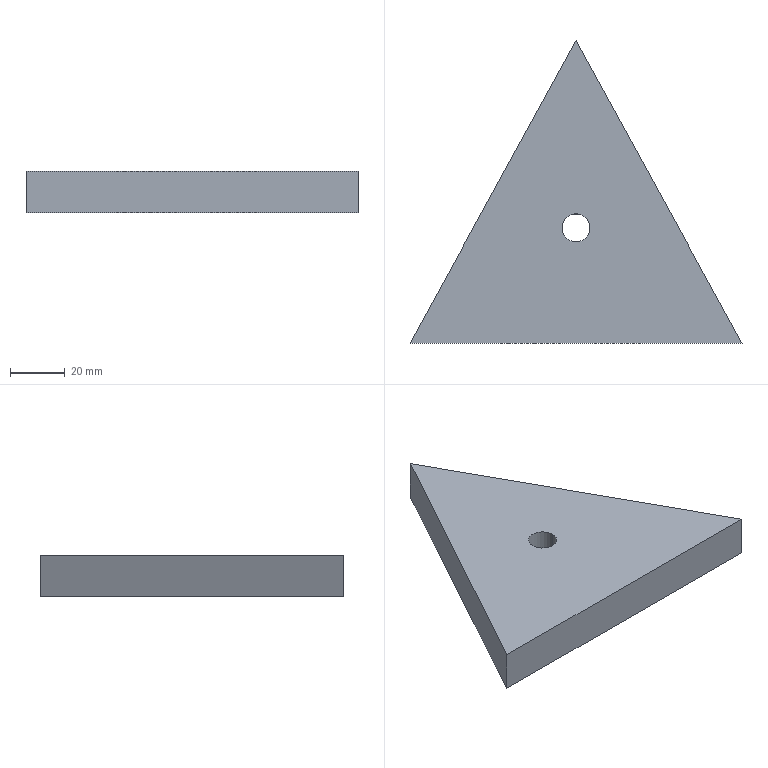Part | SolidWorks | features Extrusion 1, HoleWzd 1 | 1 solid | 7 faces | box 121 x 110.14 x 15 mm | volume 98726 mm3 | plane 5 | cylinder 2 | commonest cylinder face diameters 10.2 x2
STEP:
#1=CARTESIAN_POINT('',(5.1,-68.14,0.));
#2=VERTEX_POINT('',#1);
#3=CARTESIAN_POINT('',(-5.1,-68.14,0.));
#4=VERTEX_POINT('',#3);
#5=CARTESIAN_POINT('',(0.,-68.14,0.));
#6=DIRECTION('',(0.,0.,-1.));
#7=DIRECTION('',(-1.,0.,0.));
#8=AXIS2_PLACEMENT_3D('',#5,#6,#7);
#9=CIRCLE('',#8,5.1);
#10=EDGE_CURVE('',#2,#4,#9,.T.);
#11=ORIENTED_EDGE('',*,*,#10,.T.);
#12=CARTESIAN_POINT('',(-5.1,-68.14,15.));
#13=VERTEX_POINT('',#12);
#14=CARTESIAN_POINT('',(-5.1,-68.14,15.));
#15=DIRECTION('',(0.,0.,1.));
#16=VECTOR('',#15,1000.);
#17=LINE('',#14,#16);
#18=EDGE_CURVE('',#4,#13,#17,.T.);
#19=ORIENTED_EDGE('',*,*,#18,.T.);
#20=CARTESIAN_POINT('',(5.1,-68.14,15.));
#21=VERTEX_POINT('',#20);
#22=CARTESIAN_POINT('',(0.,-68.14,15.));
#23=DIRECTION('',(0.,0.,1.));
#24=DIRECTION('',(1.,0.,0.));
#25=AXIS2_PLACEMENT_3D('',#22,#23,#24);
#26=CIRCLE('',#25,5.1);
#27=EDGE_CURVE('',#13,#21,#26,.T.);
#28=ORIENTED_EDGE('',*,*,#27,.T.);
#29=CARTESIAN_POINT('',(5.1,-68.14,15.));
#30=DIRECTION('',(0.,0.,1.));
#31=VECTOR('',#30,1000.);
#32=LINE('',#29,#31);
#33=EDGE_CURVE('',#2,#21,#32,.T.);
#34=ORIENTED_EDGE('',*,*,#33,.F.);
#35=EDGE_LOOP('',(#11,#19,#28,#34));
#36=FACE_OUTER_BOUND('',#35,.T.);
#37=CARTESIAN_POINT('',(0.,-68.14,15.));
#38=DIRECTION('',(0.,0.,1.));
#39=DIRECTION('',(1.,0.,0.));
#40=AXIS2_PLACEMENT_3D('',#37,#38,#39);
#41=CYLINDRICAL_SURFACE('',#40,5.1);
#42=ADVANCED_FACE('',(#36),#41,.F.);
#43=CARTESIAN_POINT('',(0.,-68.14,15.));
#44=DIRECTION('',(0.,0.,1.));
#45=DIRECTION('',(1.,0.,0.));
#46=AXIS2_PLACEMENT_3D('',#43,#44,#45);
#47=CIRCLE('',#46,5.1);
#48=EDGE_CURVE('',#21,#13,#47,.T.);
#49=ORIENTED_EDGE('',*,*,#48,.F.);
#50=ORIENTED_EDGE('',*,*,#27,.F.);
#51=EDGE_LOOP('',(#49,#50));
#52=FACE_BOUND('',#51,.T.);
#53=CARTESIAN_POINT('',(60.5,-110.14,15.));
#54=VERTEX_POINT('',#53);
#55=CARTESIAN_POINT('',(0.,0.,15.));
#56=VERTEX_POINT('',#55);
#57=CARTESIAN_POINT('',(60.5,-110.14,15.));
#58=DIRECTION('',(-0.4814,0.8765,0.));
#59=VECTOR('',#58,1000.);
#60=LINE('',#57,#59);
#61=EDGE_CURVE('',#54,#56,#60,.T.);
#62=ORIENTED_EDGE('',*,*,#61,.T.);
#63=CARTESIAN_POINT('',(-60.5,-110.14,15.));
#64=VERTEX_POINT('',#63);
#65=CARTESIAN_POINT('',(0.,0.,15.));
#66=DIRECTION('',(-0.4814,-0.8765,0.));
#67=VECTOR('',#66,1000.);
#68=LINE('',#65,#67);
#69=EDGE_CURVE('',#56,#64,#68,.T.);
#70=ORIENTED_EDGE('',*,*,#69,.T.);
#71=CARTESIAN_POINT('',(-60.5,-110.14,15.));
#72=DIRECTION('',(1.,0.,0.));
#73=VECTOR('',#72,1000.);
#74=LINE('',#71,#73);
#75=EDGE_CURVE('',#64,#54,#74,.T.);
#76=ORIENTED_EDGE('',*,*,#75,.T.);
#77=EDGE_LOOP('',(#62,#70,#76));
#78=FACE_OUTER_BOUND('',#77,.T.);
#79=CARTESIAN_POINT('',(0.,0.,15.));
#80=DIRECTION('',(0.,0.,-1.));
#81=DIRECTION('',(-1.,0.,0.));
#82=AXIS2_PLACEMENT_3D('',#79,#80,#81);
#83=PLANE('',#82);
#84=ADVANCED_FACE('',(#52,#78),#83,.F.);
#85=ORIENTED_EDGE('',*,*,#10,.F.);
#86=CARTESIAN_POINT('',(0.,-68.14,0.));
#87=DIRECTION('',(0.,0.,-1.));
#88=DIRECTION('',(-1.,0.,0.));
#89=AXIS2_PLACEMENT_3D('',#86,#87,#88);
#90=CIRCLE('',#89,5.1);
#91=EDGE_CURVE('',#4,#2,#90,.T.);
#92=ORIENTED_EDGE('',*,*,#91,.F.);
#93=EDGE_LOOP('',(#85,#92));
#94=FACE_BOUND('',#93,.T.);
#95=CARTESIAN_POINT('',(60.5,-110.14,0.));
#96=VERTEX_POINT('',#95);
#97=CARTESIAN_POINT('',(0.,0.,0.));
#98=VERTEX_POINT('',#97);
#99=CARTESIAN_POINT('',(60.5,-110.14,0.));
#100=DIRECTION('',(-0.4814,0.8765,0.));
#101=VECTOR('',#100,1000.);
#102=LINE('',#99,#101);
#103=EDGE_CURVE('',#96,#98,#102,.T.);
#104=ORIENTED_EDGE('',*,*,#103,.F.);
#105=CARTESIAN_POINT('',(-60.5,-110.14,0.));
#106=VERTEX_POINT('',#105);
#107=CARTESIAN_POINT('',(-60.5,-110.14,0.));
#108=DIRECTION('',(1.,0.,0.));
#109=VECTOR('',#108,1000.);
#110=LINE('',#107,#109);
#111=EDGE_CURVE('',#106,#96,#110,.T.);
#112=ORIENTED_EDGE('',*,*,#111,.F.);
#113=CARTESIAN_POINT('',(0.,0.,0.));
#114=DIRECTION('',(-0.4814,-0.8765,0.));
#115=VECTOR('',#114,1000.);
#116=LINE('',#113,#115);
#117=EDGE_CURVE('',#98,#106,#116,.T.);
#118=ORIENTED_EDGE('',*,*,#117,.F.);
#119=EDGE_LOOP('',(#104,#112,#118));
#120=FACE_OUTER_BOUND('',#119,.T.);
#121=CARTESIAN_POINT('',(0.,0.,0.));
#122=DIRECTION('',(0.,0.,-1.));
#123=DIRECTION('',(-1.,0.,0.));
#124=AXIS2_PLACEMENT_3D('',#121,#122,#123);
#125=PLANE('',#124);
#126=ADVANCED_FACE('',(#94,#120),#125,.T.);
#127=ORIENTED_EDGE('',*,*,#103,.T.);
#128=CARTESIAN_POINT('',(0.,0.,15.));
#129=DIRECTION('',(0.,0.,-1.));
#130=VECTOR('',#129,1000.);
#131=LINE('',#128,#130);
#132=EDGE_CURVE('',#56,#98,#131,.T.);
#133=ORIENTED_EDGE('',*,*,#132,.F.);
#134=ORIENTED_EDGE('',*,*,#61,.F.);
#135=CARTESIAN_POINT('',(60.5,-110.14,15.));
#136=DIRECTION('',(0.,0.,-1.));
#137=VECTOR('',#136,1000.);
#138=LINE('',#135,#137);
#139=EDGE_CURVE('',#54,#96,#138,.T.);
#140=ORIENTED_EDGE('',*,*,#139,.T.);
#141=EDGE_LOOP('',(#127,#133,#134,#140));
#142=FACE_OUTER_BOUND('',#141,.T.);
#143=CARTESIAN_POINT('',(60.5,-110.14,15.));
#144=DIRECTION('',(-0.8765,-0.4814,0.));
#145=DIRECTION('',(0.4814,-0.8765,0.));
#146=AXIS2_PLACEMENT_3D('',#143,#144,#145);
#147=PLANE('',#146);
#148=ADVANCED_FACE('',(#142),#147,.F.);
#149=ORIENTED_EDGE('',*,*,#117,.T.);
#150=CARTESIAN_POINT('',(-60.5,-110.14,15.));
#151=DIRECTION('',(0.,0.,-1.));
#152=VECTOR('',#151,1000.);
#153=LINE('',#150,#152);
#154=EDGE_CURVE('',#64,#106,#153,.T.);
#155=ORIENTED_EDGE('',*,*,#154,.F.);
#156=ORIENTED_EDGE('',*,*,#69,.F.);
#157=ORIENTED_EDGE('',*,*,#132,.T.);
#158=EDGE_LOOP('',(#149,#155,#156,#157));
#159=FACE_OUTER_BOUND('',#158,.T.);
#160=CARTESIAN_POINT('',(0.,0.,15.));
#161=DIRECTION('',(0.8765,-0.4814,0.));
#162=DIRECTION('',(0.4814,0.8765,0.));
#163=AXIS2_PLACEMENT_3D('',#160,#161,#162);
#164=PLANE('',#163);
#165=ADVANCED_FACE('',(#159),#164,.F.);
#166=ORIENTED_EDGE('',*,*,#111,.T.);
#167=ORIENTED_EDGE('',*,*,#139,.F.);
#168=ORIENTED_EDGE('',*,*,#75,.F.);
#169=ORIENTED_EDGE('',*,*,#154,.T.);
#170=EDGE_LOOP('',(#166,#167,#168,#169));
#171=FACE_OUTER_BOUND('',#170,.T.);
#172=CARTESIAN_POINT('',(-60.5,-110.14,15.));
#173=DIRECTION('',(0.,1.,0.));
#174=DIRECTION('',(0.,0.,1.));
#175=AXIS2_PLACEMENT_3D('',#172,#173,#174);
#176=PLANE('',#175);
#177=ADVANCED_FACE('',(#171),#176,.F.);
#178=ORIENTED_EDGE('',*,*,#18,.F.);
#179=ORIENTED_EDGE('',*,*,#91,.T.);
#180=ORIENTED_EDGE('',*,*,#33,.T.);
#181=ORIENTED_EDGE('',*,*,#48,.T.);
#182=EDGE_LOOP('',(#178,#179,#180,#181));
#183=FACE_OUTER_BOUND('',#182,.T.);
#184=CARTESIAN_POINT('',(0.,-68.14,15.));
#185=DIRECTION('',(0.,0.,1.));
#186=DIRECTION('',(1.,0.,0.));
#187=AXIS2_PLACEMENT_3D('',#184,#185,#186);
#188=CYLINDRICAL_SURFACE('',#187,5.1);
#189=ADVANCED_FACE('',(#183),#188,.F.);
#190=CLOSED_SHELL('',(#42,#84,#126,#148,#165,#177,#189));
#191=MANIFOLD_SOLID_BREP('',#190);
#192=CARTESIAN_POINT('',(0.,0.,0.));
#193=DIRECTION('',(0.,0.,1.));
#194=DIRECTION('',(1.,0.,0.));
#195=AXIS2_PLACEMENT_3D('',#192,#193,#194);
#196=(LENGTH_UNIT()NAMED_UNIT(*)SI_UNIT(.MILLI.,.METRE.));
#197=UNCERTAINTY_MEASURE_WITH_UNIT(LENGTH_MEASURE(0.00001),#196,'','');
#198=(NAMED_UNIT(*)PLANE_ANGLE_UNIT()SI_UNIT($,.RADIAN.));
#199=(NAMED_UNIT(*)SI_UNIT($,.STERADIAN.)SOLID_ANGLE_UNIT());
#200=(GEOMETRIC_REPRESENTATION_CONTEXT(3)GLOBAL_UNCERTAINTY_ASSIGNED_CONTEXT((#197))GLOBAL_UNIT_ASSIGNED_CONTEXT((#196,#198,#199))REPRESENTATION_CONTEXT('',''));
#201=ADVANCED_BREP_SHAPE_REPRESENTATION('',(#191,#195),#200);